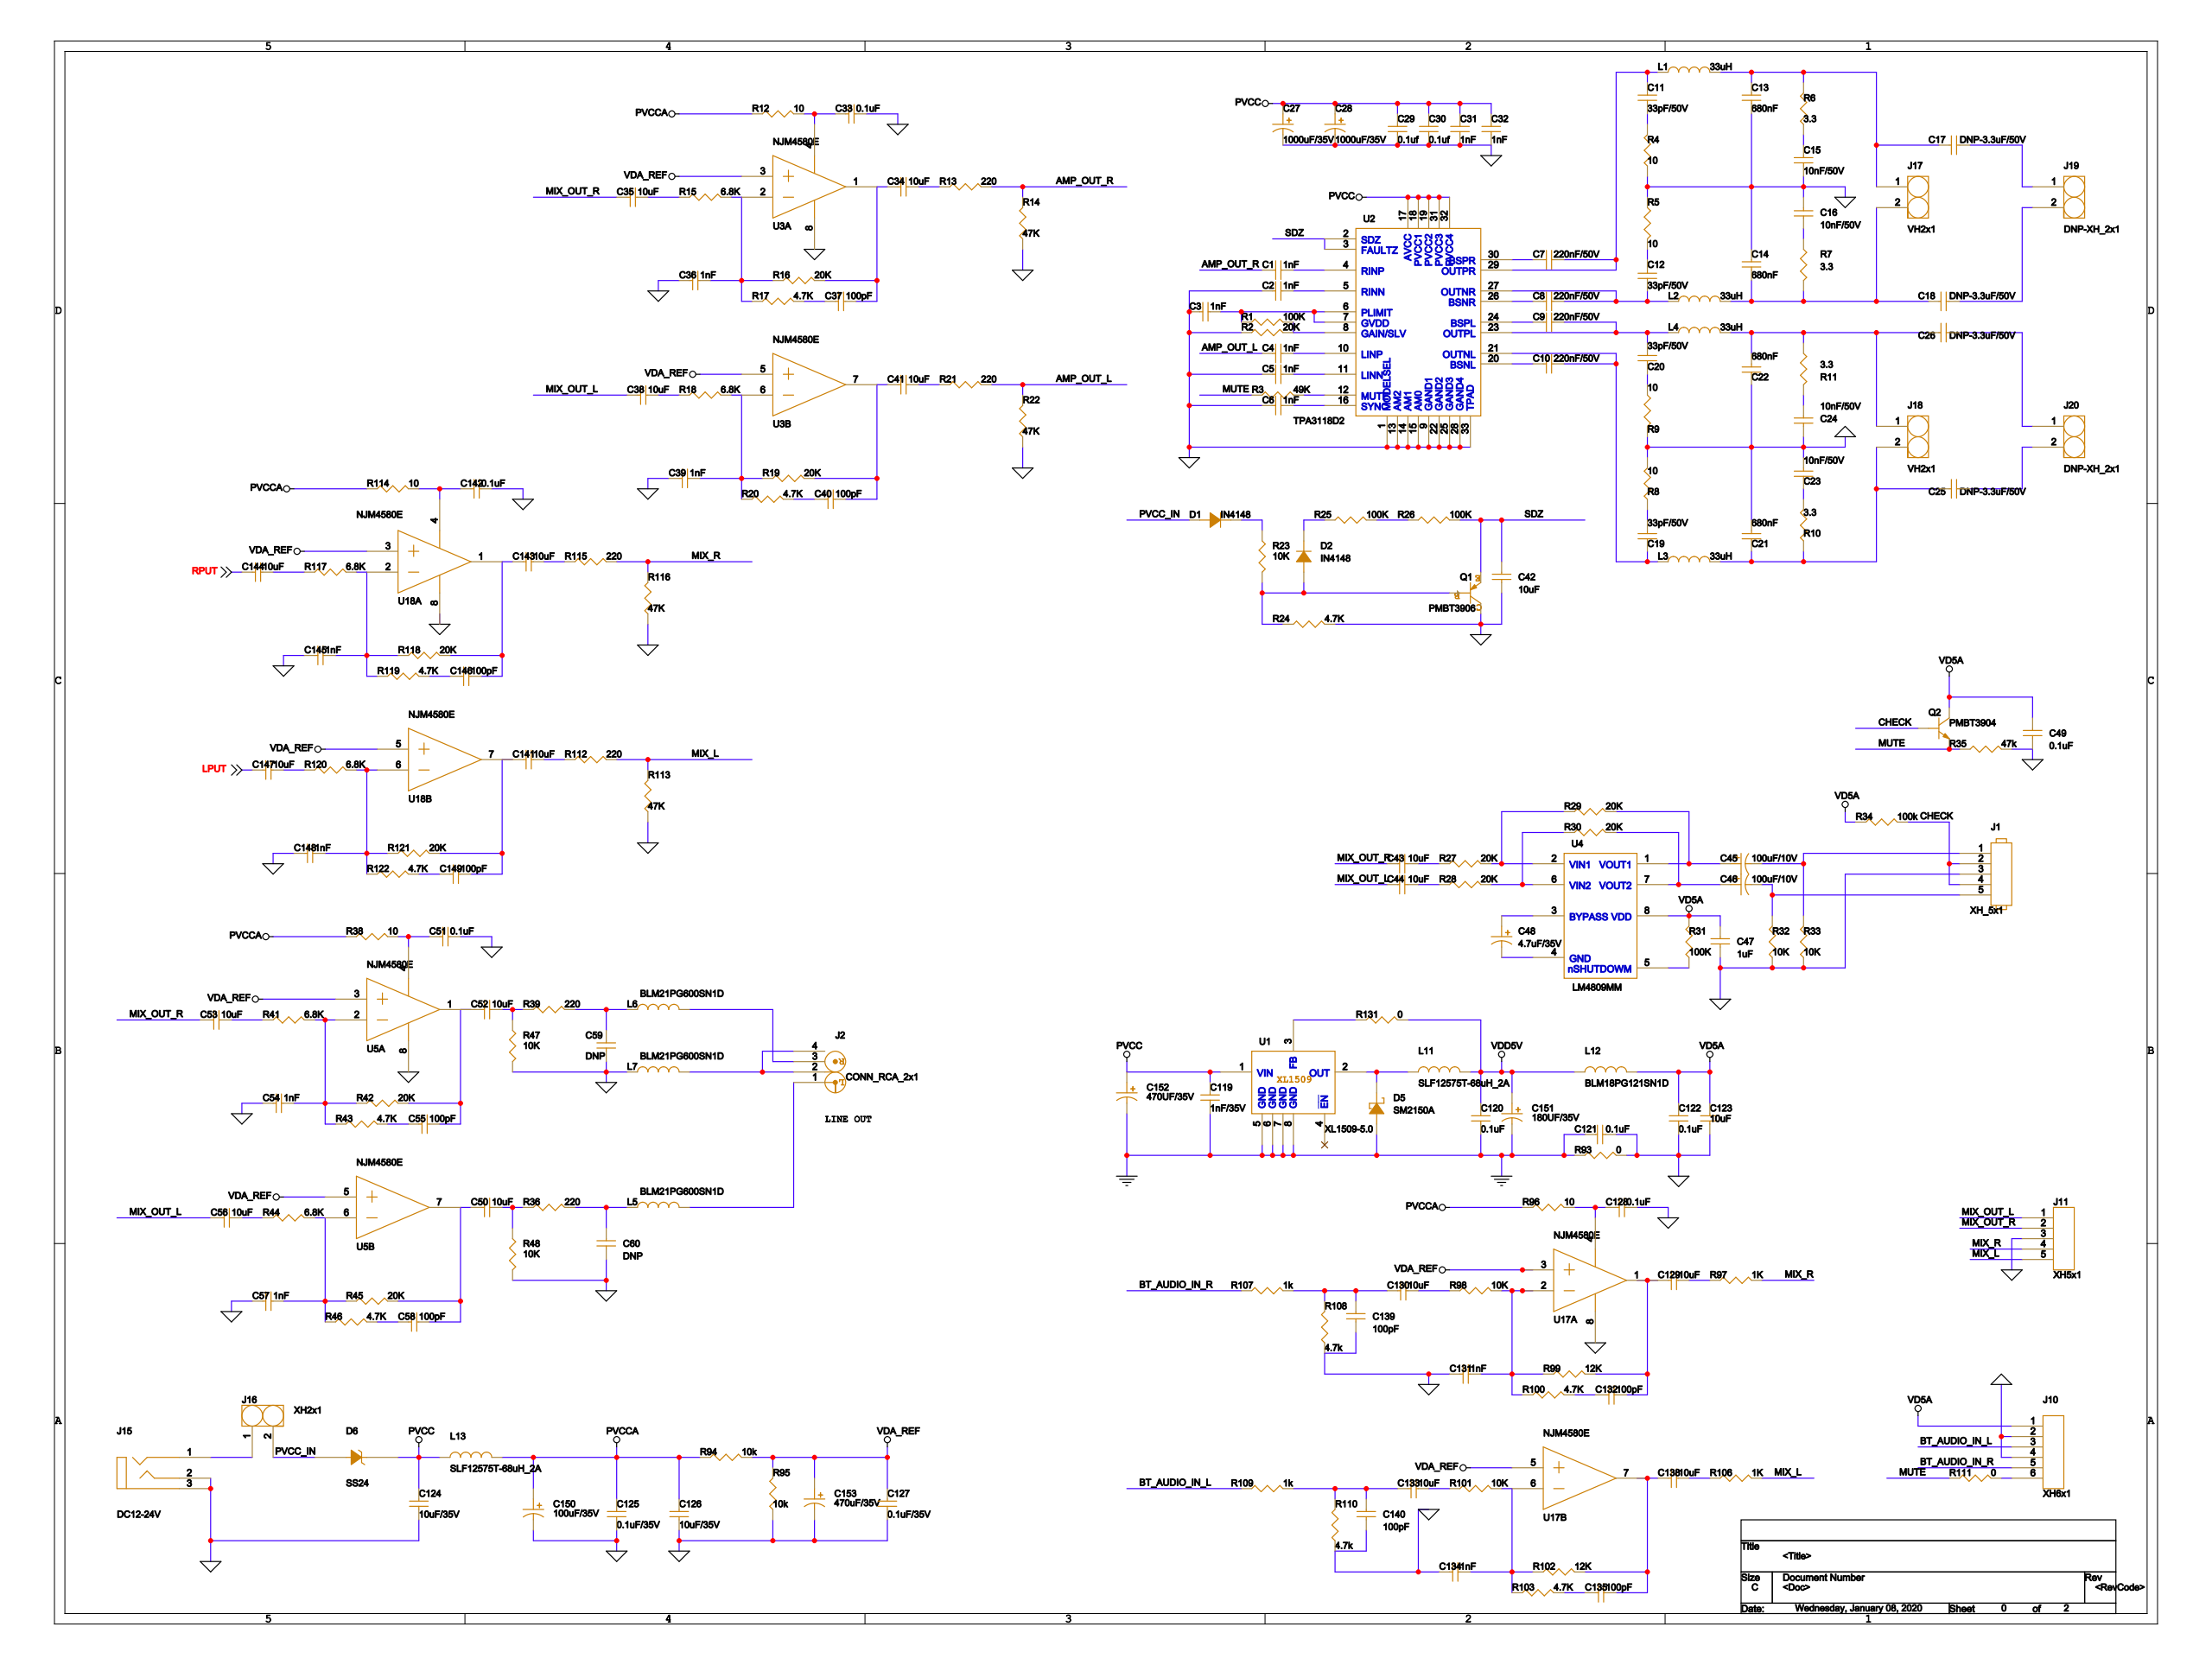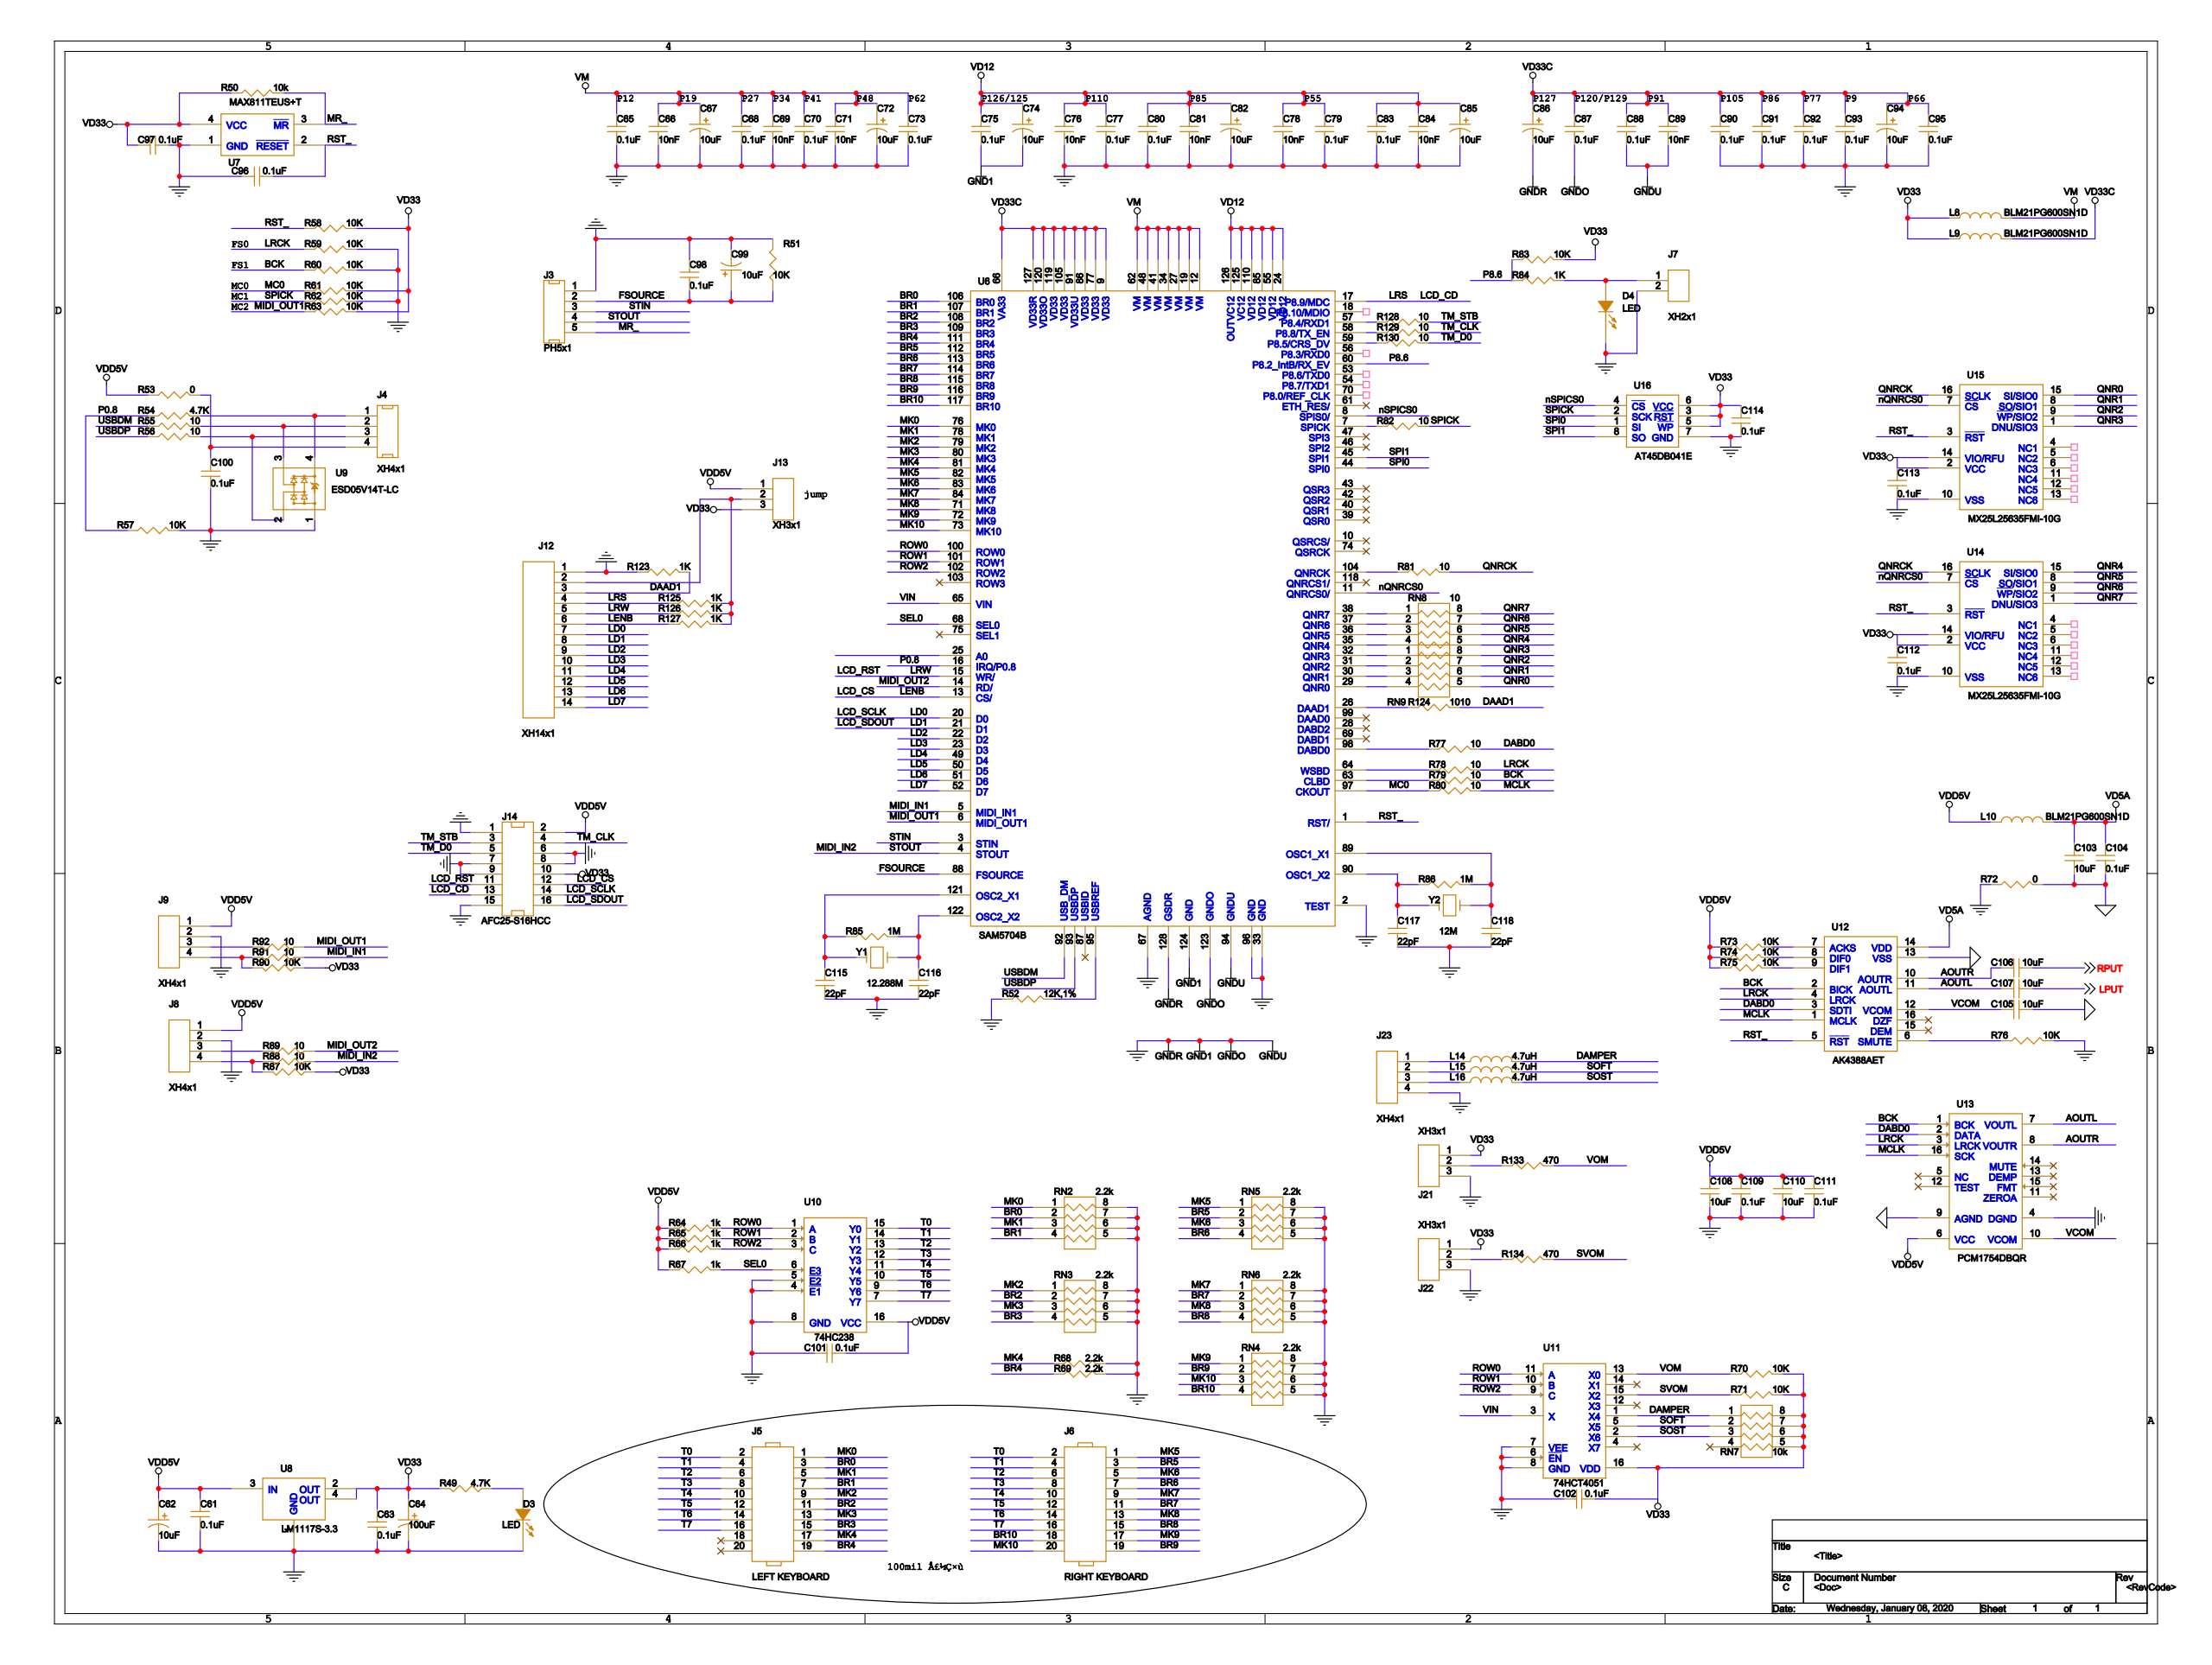Circuit board | Cadence Allegro | 355 parts | 259 nets
Bill of materials:
SYM_NAME,COMP_DEVICE_TYPE,COMP_VALUE,COMP_TOL,COMP_CLASS,REFDES
C0603,CAP NP_C0603_1NF,1nF,,IC,C1
C0603,CAP NP_C0603_1NF,1nF,,IC,C2
C0603,CAP NP_C0603_1NF,1nF,,IC,C3
C0603,CAP NP_C0603_1NF,1nF,,IC,C4
C0603,CAP NP_C0603_1NF,1nF,,IC,C5
C0603,CAP NP_C0603_1NF,1nF,,IC,C6
C0603,CAP NP_C0603_220NF/50V,220nF/50V,,IC,C7
C0603,CAP NP_C0603_220NF/50V,220nF/50V,,IC,C8
C0603,CAP NP_C0603_220NF/50V,220nF/50V,,IC,C9
C0603,CAP NP_C0603_220NF/50V,220nF/50V,,IC,C10
C0603,CAP NP_C0603_33PF/50V,33pF/50V,,IC,C11
C0603,CAP NP_C0603_33PF/50V,33pF/50V,,IC,C12
C0603,CAP NP_C0603_680NF,680nF,,IC,C13
C0603,CAP NP_C0603_680NF,680nF,,IC,C14
C0603,CAP NP_C0603_10NF/50V,10nF/50V,,IC,C15
C0603,CAP NP_C0603_10NF/50V,10nF/50V,,IC,C16
C0603,CAP NP_C0603_DNP-3.3UF/50V,DNP-3.3uF/50V,,IC,C17
C0603,CAP NP_C0603_DNP-3.3UF/50V,DNP-3.3uF/50V,,IC,C18
C0603,CAP NP_C0603_33PF/50V,33pF/50V,,IC,C19
C0603,CAP NP_C0603_33PF/50V,33pF/50V,,IC,C20
C0603,CAP NP_C0603_680NF,680nF,,IC,C21
C0603,CAP NP_C0603_680NF,680nF,,IC,C22
C0603,CAP NP_C0603_10NF/50V,10nF/50V,,IC,C23
C0603,CAP NP_C0603_10NF/50V,10nF/50V,,IC,C24
C0603,CAP NP_C0603_DNP-3.3UF/50V,DNP-3.3uF/50V,,IC,C25
C0603,CAP NP_C0603_DNP-3.3UF/50V,DNP-3.3uF/50V,,IC,C26
CAP_13X20MM,CAP POL_CAP_13X20MM_1000UF/35V,1000uF/35V,,IC,C27
CAP_13X20MM,CAP POL_CAP_13X20MM_1000UF/35V,1000uF/35V,,IC,C28
C0603,CAP NP_C0603_0.1UF,0.1uF,,IC,C29
C0603,CAP NP_C0603_0.1UF,0.1uF,,IC,C30
C0603,CAP NP_C0603_1NF,1nF,,IC,C31
C0603,CAP NP_C0603_1NF,1nF,,IC,C32
C0603,CAP NP_C0603_0.1UF,0.1uF,,IC,C33
C0805,CAP NP_C0805_10UF,10uF,,IC,C34
C0805,CAP NP_C0805_10UF,10uF,,IC,C35
C0603,CAP NP_C0603_1NF,1nF,,IC,C36
C0603,CAP NP_C0603_100PF,100pF,,IC,C37
C0805,CAP NP_C0805_10UF,10uF,,IC,C38
C0603,CAP NP_C0603_1NF,1nF,,IC,C39
C0603,CAP NP_C0603_100PF,100pF,,IC,C40
C0805,CAP NP_C0805_10UF,10uF,,IC,C41
C0805,CAP NP_C0805_10UF,10uF,,IC,C42
C0805,CAP NP_C0805_10UF,10uF,,IC,C43
C0805,CAP NP_C0805_10UF,10uF,,IC,C44
CAP_6P3X11MM,CAP POL_CAP_6P3X11MM_100UF/10V,100uF/10V,,IC,C45
CAP_6P3X11MM,CAP POL_CAP_6P3X11MM_100UF/10V,100uF/10V,,IC,C46
C0603,CAP NP_C0603_1UF,1uF,,IC,C47
CAP_4X7MM,CAP POL_CAP_4X7MM_4.7UF/35V,4.7uF/35V,,IC,C48
C0603,CAP NP_C0603_0.1UF,0.1uF,,IC,C49
C0805,CAP NP_C0805_10UF,10uF,,IC,C50
C0603,CAP NP_C0603_0.1UF,0.1uF,,IC,C51
C0805,CAP NP_C0805_10UF,10uF,,IC,C52
C0805,CAP NP_C0805_10UF,10uF,,IC,C53
C0603,CAP NP_C0603_1NF,1nF,,IC,C54
C0603,CAP NP_C0603_100PF,100pF,,IC,C55
C0805,CAP NP_C0805_10UF,10uF,,IC,C56
C0603,CAP NP_C0603_1NF,1nF,,IC,C57
C0603,CAP NP_C0603_100PF,100pF,,IC,C58
C0603,CAP NP_C0603_DNP,DNP,,IC,C59
C0603,CAP NP_C0603_DNP,DNP,,IC,C60
C0603,CAP NP_C0603_0.1UF,0.1uF,,IC,C61
C0805,CAP POL_C0805_10UF,10uF,,IC,C62
C0603,CAP NP_C0603_0.1UF,0.1uF,,IC,C63
CAP_6P3X11MM,CAP POL_CAP_6P3X11MM_100UF,100uF,,IC,C64
C0603,CAP NP_C0603_0.1UF,0.1uF,,IC,C65
C0603,CAP NP_C0603_10NF,10nF,,IC,C66
C0805,CAP POL_C0805_10UF,10uF,,IC,C67
C0603,CAP NP_C0603_0.1UF,0.1uF,,IC,C68
C0603,CAP NP_C0603_10NF,10nF,,IC,C69
C0603,CAP NP_C0603_0.1UF,0.1uF,,IC,C70
C0603,CAP NP_C0603_10NF,10nF,,IC,C71
C0805,CAP POL_C0805_10UF,10uF,,IC,C72
C0603,CAP NP_C0603_0.1UF,0.1uF,,IC,C73
C0805,CAP POL_C0805_10UF,10uF,,IC,C74
C0603,CAP NP_C0603_0.1UF,0.1uF,,IC,C75
C0603,CAP NP_C0603_10NF,10nF,,IC,C76
C0603,CAP NP_C0603_0.1UF,0.1uF,,IC,C77
C0603,CAP NP_C0603_10NF,10nF,,IC,C78
C0603,CAP NP_C0603_0.1UF,0.1uF,,IC,C79
C0603,CAP NP_C0603_0.1UF,0.1uF,,IC,C80
C0603,CAP NP_C0603_10NF,10nF,,IC,C81
C0805,CAP POL_C0805_10UF,10uF,,IC,C82
C0603,CAP NP_C0603_0.1UF,0.1uF,,IC,C83
C0603,CAP NP_C0603_10NF,10nF,,IC,C84
C0805,CAP POL_C0805_10UF,10uF,,IC,C85
C0805,CAP POL_C0805_10UF,10uF,,IC,C86
C0603,CAP NP_C0603_0.1UF,0.1uF,,IC,C87
C0603,CAP NP_C0603_0.1UF,0.1uF,,IC,C88
C0603,CAP NP_C0603_10NF,10nF,,IC,C89
C0603,CAP NP_C0603_0.1UF,0.1uF,,IC,C90
C0603,CAP NP_C0603_0.1UF,0.1uF,,IC,C91
C0603,CAP NP_C0603_0.1UF,0.1uF,,IC,C92
C0603,CAP NP_C0603_0.1UF,0.1uF,,IC,C93
C0805,CAP POL_C0805_10UF,10uF,,IC,C94
C0603,CAP NP_C0603_0.1UF,0.1uF,,IC,C95
C0603,CAP NP_C0603_0.1UF,0.1uF,,IC,C96
C0603,CAP NP_C0603_0.1UF,0.1uF,,IC,C97
C0603,CAP NP_C0603_0.1UF,0.1uF,,IC,C98
C0805,CAP POL_C0805_10UF,10uF,,IC,C99
C0603,CAP NP_C0603_0.1UF,0.1uF,,IC,C100
C0603,CAP NP_C0603_0.1UF,0.1uF,,IC,C101
C0603,CAP NP_C0603_0.1UF,0.1uF,,IC,C102
C0805,CAP NP_C0805_10UF,10uF,,IC,C103
C0603,CAP NP_C0603_0.1UF,0.1uF,,IC,C104
C0805,CAP NP_C0805_10UF,10uF,,IC,C105
C0805,CAP NP_C0805_10UF,10uF,,IC,C106
C0805,CAP NP_C0805_10UF,10uF,,IC,C107
C0805,CAP NP_C0805_10UF,10uF,,IC,C108
C0603,CAP NP_C0603_0.1UF,0.1uF,,IC,C109
C0805,CAP NP_C0805_10UF,10uF,,IC,C110
C0603,CAP NP_C0603_0.1UF,0.1uF,,IC,C111
C0603,CAP NP_C0603_0.1UF,0.1uF,,IC,C112
C0603,CAP NP_C0603_0.1UF,0.1uF,,IC,C113
C0603,CAP NP_C0603_0.1UF,0.1uF,,IC,C114
C0603,CAP NP_C0603_22PF,22pF,,IC,C115
C0603,CAP NP_C0603_22PF,22pF,,IC,C116
C0603,CAP NP_C0603_22PF,22pF,,IC,C117
C0603,CAP NP_C0603_22PF,22pF,,IC,C118
C0603,CAP NP_C0603_1NF/35V,1nF/35V,,IC,C119
C0603,CAP NP_C0603_0.1UF,0.1uF,,IC,C120
C0603,CAP NP_C0603_0.1UF,0.1uF,,IC,C121
C0603,CAP NP_C0603_0.1UF,0.1uF,,IC,C122
C0805,CAP NP_C0805_10UF,10uF,,IC,C123
C0805,CAP NP_C0805_10UF/35V,10uF/35V,,IC,C124
C0603,CAP NP_C0603_0.1UF/35V,0.1uF/35V,,IC,C125
C0805,CAP NP_C0805_10UF/35V,10uF/35V,,IC,C126
C0603,CAP NP_C0603_0.1UF/35V,0.1uF/35V,,IC,C127
C0603,CAP NP_C0603_0.1UF,0.1uF,,IC,C128
C0805,CAP NP_C0805_10UF,10uF,,IC,C129
C0805,CAP NP_C0805_10UF,10uF,,IC,C130
C0603,CAP NP_C0603_1NF,1nF,,IC,C131
C0603,CAP NP_C0603_100PF,100pF,,IC,C132
C0805,CAP NP_C0805_10UF,10uF,,IC,C133
C0603,CAP NP_C0603_1NF,1nF,,IC,C134
C0603,CAP NP_C0603_100PF,100pF,,IC,C135
C0805,CAP NP_C0805_10UF,10uF,,IC,C138
C0603,CAP NP_C0603_100PF,100pF,,IC,C139
C0603,CAP NP_C0603_100PF,100pF,,IC,C140
C0805,CAP NP_C0805_10UF,10uF,,IC,C141
C0603,CAP NP_C0603_0.1UF,0.1uF,,IC,C142
C0805,CAP NP_C0805_10UF,10uF,,IC,C143
C0805,CAP NP_C0805_10UF,10uF,,IC,C144
C0603,CAP NP_C0603_1NF,1nF,,IC,C145
C0603,CAP NP_C0603_100PF,100pF,,IC,C146
C0805,CAP NP_C0805_10UF,10uF,,IC,C147
C0603,CAP NP_C0603_1NF,1nF,,IC,C148
C0603,CAP NP_C0603_100PF,100pF,,IC,C149
CAP_6P3X11MM,CAP POL_CAP_6P3X11MM_100UF/35V,100uF/35V,,IC,C150
CAP_6P3X11MM,CAP POL_CAP_6P3X11MM_180UF/35V,180UF/35V,,IC,C151
CAP_10X17MM,CAP POL_CAP_10X17MM_470UF/35V,470UF/35V,,IC,C152
CAP_10X17MM,CAP POL_CAP_10X17MM_470UF/35V,470UF/35V,,IC,C153
SOD-123,DIODE_SOD-123_IN4148,IN4148,,IC,D1
SOD-123,DIODE_SOD-123_IN4148,IN4148,,IC,D2
LED0805,LED_0_LED0805_LED,LED,,IC,D3
LED0805,LED_0_LED0805_LED,LED,,IC,D4
SMA-FL,SGL41/SM_SMA-FL_SM2150A,SM2150A,,IC,D5
DO-214AC_5P28X2P9M,ICL8069/SO_0_DO-214AC_5P28X2P9M,SS24,,IC,D6
XH-5A,HEADER 5_XH-5A_XH_5X1,XH_5x1,,IC,J1
XH-4A,CONN_RCA_0_XH-4A_CONN_RCA_2X1,CONN_RCA_2x1,,IC,J2
PH-5A,CONN RECT 5_PH-5A_PH5X1,PH5x1,,IC,J3
XH-4A,CONN PCB 4-R_XH-4A_XH4X1,XH4x1,,IC,J4
IDC10X2,HEADER 10X2_IDC10X2_LEFT KEYBOA,LEFT KEYBOARD,,IC,J5
IDC10X2,HEADER 10X2_IDC10X2_RIGHT KEYBO,RIGHT KEYBOARD,,IC,J6
XH-2A,CON2_XH-2A_XH2X1,XH2x1,,IC,J7
XH254_4_V,CON4_XH254_4_V_XH4X1,XH4x1,,IC,J8
XH254_4_V,CON4_XH254_4_V_XH4X1,XH4x1,,IC,J9
XH-6A,CON6_XH-6A_XH6X1,XH6x1,,IC,J10
XH-5A,CON5_XH-5A_XH5X1,XH5x1,,IC,J11
XH254_14_V,CON14_XH254_14_V_XH14X1,XH14x1,,IC,J12
XH-3A,CON3_XH-3A_XH3X1,XH3x1,,IC,J13
FPC_1P25MM16P,CONN PCB 8X2-R_FPC_1P25MM16P_AF,AFC25-S16HCC,,IC,J14
DC-0055P5-2P0MM,PHONEJACK STEREO_DC-0055P5-2P0M,DC12-24V,,IC,J15
XH-2A,XH2X1_XH-2A_XH2X1,XH2x1,,IC,J16
VH-2A,XH2X1_VH-2A_VH2X1,VH2x1,,IC,J17
VH-2A,XH2X1_VH-2A_VH2X1,VH2x1,,IC,J18
XH-2A,XH2X1_XH-2A_DNP-XH_2X1,DNP-XH_2x1,,IC,J19
XH-2A,XH2X1_XH-2A_DNP-XH_2X1,DNP-XH_2x1,,IC,J20
XH-3A,CON3_XH-3A_XH3X1,XH3x1,,IC,J21
XH-3A,CON3_XH-3A_XH3X1,XH3x1,,IC,J22
XH254_4_V,CON4_XH254_4_V_XH4X1,XH4x1,,IC,J23
L_12P5X12P5X7P5MM,INDUCTOR_L_12P5X12P5X7P5MM_33UH,33uH,,IC,L1
L_12P5X12P5X7P5MM,INDUCTOR_L_12P5X12P5X7P5MM_33UH,33uH,,IC,L2
L_12P5X12P5X7P5MM,INDUCTOR_L_12P5X12P5X7P5MM_33UH,33uH,,IC,L3
L_12P5X12P5X7P5MM,INDUCTOR_L_12P5X12P5X7P5MM_33UH,33uH,,IC,L4
L0603,INDUCTOR_L0603_ BLM21PG600SN1D,BLM21PG600SN1D,,IC,L5
L0603,INDUCTOR_L0603_ BLM21PG600SN1D,BLM21PG600SN1D,,IC,L6
L0603,INDUCTOR_L0603_ BLM21PG600SN1D,BLM21PG600SN1D,,IC,L7
L0805,INDUCTOR_L0805_ BLM21PG600SN1D,BLM21PG600SN1D,,IC,L8
L0805,INDUCTOR_L0805_ BLM21PG600SN1D,BLM21PG600SN1D,,IC,L9
L0805,INDUCTOR_L0805_ BLM21PG600SN1D,BLM21PG600SN1D,,IC,L10
L_12P5X12P5X7P5MM,INDUCTOR_L_12P5X12P5X7P5MM_SLF1,SLF12575T-68uH_2A,,IC,L11
L0603,INDUCTOR_L0603_BLM18PG121SN1D,BLM18PG121SN1D,,IC,L12
L_12P5X12P5X7P5MM,INDUCTOR_L_12P5X12P5X7P5MM_SLF1,SLF12575T-68uH_2A,,IC,L13
L0805,INDUCTOR_L0805_4.7UH,4.7uH,,IC,L14
L0805,INDUCTOR_L0805_4.7UH,4.7uH,,IC,L15
L0805,INDUCTOR_L0805_4.7UH,4.7uH,,IC,L16
SOT-23,PMBT3906_0_SOT-23_PMBT3906,PMBT3906,,IC,Q1
SOT-23,PMBT3904_0_SOT-23_PMBT3904,PMBT3904,,IC,Q2
R0603,R_R0603_100K,100K,,IC,R1
R0603,R_R0603_20K,20K,,IC,R2
R0603,R_R0603_49K,49K,,IC,R3
R0603,R_R0603_10,10,,IC,R4
R0603,R_R0603_10,10,,IC,R5
R0603,R_R0603_3.3,3.3,,IC,R6
R0603,R_R0603_3.3,3.3,,IC,R7
R0603,R_R0603_10,10,,IC,R8
R0603,R_R0603_10,10,,IC,R9
R0603,R_R0603_3.3,3.3,,IC,R10
R0603,R_R0603_3.3,3.3,,IC,R11
R0603,R_R0603_10,10,,IC,R12
R0603,R_R0603_220,220,,IC,R13
R0603,R_R0603_47K,47K,,IC,R14
R0603,R_R0603_6.8K,6.8K,,IC,R15
R0603,R_R0603_20K,20K,,IC,R16
R0603,R_R0603_4.7K,4.7K,,IC,R17
R0603,R_R0603_6.8K,6.8K,,IC,R18
R0603,R_R0603_20K,20K,,IC,R19
R0603,R_R0603_4.7K,4.7K,,IC,R20
R0603,R_R0603_220,220,,IC,R21
R0603,R_R0603_47K,47K,,IC,R22
R0603,R_R0603_10K,10K,,IC,R23
R0603,R_R0603_4.7K,4.7K,,IC,R24
R0603,R_R0603_100K,100K,,IC,R25
R0603,R_R0603_100K,100K,,IC,R26
R0603,R_R0603_20K,20K,,IC,R27
R0603,R_R0603_20K,20K,,IC,R28
R0603,R_R0603_20K,20K,,IC,R29
R0603,R_R0603_20K,20K,,IC,R30
R0603,R_R0603_100K,100K,,IC,R31
R0603,R_R0603_10K,10K,,IC,R32
R0603,R_R0603_10K,10K,,IC,R33
R0603,R_R0603_100K,100K,,IC,R34
R0603,R_R0603_47K,47K,,IC,R35
R0603,R_R0603_220,220,,IC,R36
R0603,R_R0603_10,10,,IC,R38
R0603,R_R0603_220,220,,IC,R39
R0603,R_R0603_6.8K,6.8K,,IC,R41
R0603,R_R0603_20K,20K,,IC,R42
R0603,R_R0603_4.7K,4.7K,,IC,R43
R0603,R_R0603_6.8K,6.8K,,IC,R44
R0603,R_R0603_20K,20K,,IC,R45
R0603,R_R0603_4.7K,4.7K,,IC,R46
R0603,R_R0603_10K,10K,,IC,R47
R0603,R_R0603_10K,10K,,IC,R48
R0603,R_R0603_4.7K,4.7K,,IC,R49
R0603,R_R0603_10K,10K,,IC,R50
R0603,R_R0603_10K,10K,,IC,R51
R0603,"R_R0603_12K,1%","12K,1%",,IC,R52
R0603,R_R0603_0,0,,IC,R53
R0603,R_R0603_4.7K,4.7K,,IC,R54
R0603,R_R0603_10,10,,IC,R55
R0603,R_R0603_10,10,,IC,R56
R0603,R_R0603_10K,10K,,IC,R57
R0603,R_R0603_10K,10K,,IC,R58
R0603,R_R0603_10K,10K,,IC,R59
R0603,R_R0603_10K,10K,,IC,R60
R0603,R_R0603_10K,10K,,IC,R61
R0603,R_R0603_10K,10K,,IC,R62
R0603,R_R0603_10K,10K,,IC,R63
R0603,R_R0603_1K,1K,,IC,R64
R0603,R_R0603_1K,1K,,IC,R65
R0603,R_R0603_1K,1K,,IC,R66
R0603,R_R0603_1K,1K,,IC,R67
R0603,R_R0603_2.2K,2.2k,,IC,R68
R0603,R_R0603_2.2K,2.2k,,IC,R69
R0603,R_R0603_10K,10K,,IC,R70
R0603,R_R0603_10K,10K,,IC,R71
R0603,R_R0603_0,0,,IC,R72
R0603,R_R0603_10K,10K,,IC,R73
R0603,R_R0603_10K,10K,,IC,R74
R0603,R_R0603_10K,10K,,IC,R75
R0603,R_R0603_10K,10K,,IC,R76
R0603,R_R0603_10,10,,IC,R77
R0603,R_R0603_10,10,,IC,R78
R0603,R_R0603_10,10,,IC,R79
R0603,R_R0603_10,10,,IC,R80
R0603,R_R0603_10,10,,IC,R81
R0603,R_R0603_10,10,,IC,R82
R0603,R_R0603_10K,10K,,IC,R83
R0603,R_R0603_1K,1K,,IC,R84
R0603,R_R0603_1M,1M,,IC,R85
R0603,R_R0603_1M,1M,,IC,R86
R0603,R_R0603_10K,10K,,IC,R87
R0603,R_R0603_10,10,,IC,R88
R0603,R_R0603_10,10,,IC,R89
R0603,R_R0603_10K,10K,,IC,R90
R0603,R_R0603_10,10,,IC,R91
R0603,R_R0603_10,10,,IC,R92
R0603,R_R0603_0,0,,IC,R93
R0603,R_R0603_10K,10K,,IC,R94
R0603,R_R0603_10K,10K,,IC,R95
R0603,R_R0603_10,10,,IC,R96
R0603,R_R0603_1K,1K,,IC,R97
R0603,R_R0603_10K,10K,,IC,R98
R0603,R_R0603_12K,12K,,IC,R99
R0603,R_R0603_4.7K,4.7K,,IC,R100
R0603,R_R0603_10K,10K,,IC,R101
R0603,R_R0603_12K,12K,,IC,R102
R0603,R_R0603_4.7K,4.7K,,IC,R103
R0603,R_R0603_1K,1K,,IC,R106
R0603,R_R0603_1K,1K,,IC,R107
R0603,R_R0603_4.7K,4.7K,,IC,R108
R0603,R_R0603_1K,1K,,IC,R109
R0603,R_R0603_4.7K,4.7K,,IC,R110
R0603,R_R0603_0,0,,IC,R111
R0603,R_R0603_220,220,,IC,R112
R0603,R_R0603_47K,47K,,IC,R113
R0603,R_R0603_10,10,,IC,R114
R0603,R_R0603_220,220,,IC,R115
R0603,R_R0603_47K,47K,,IC,R116
R0603,R_R0603_6.8K,6.8K,,IC,R117
R0603,R_R0603_20K,20K,,IC,R118
R0603,R_R0603_4.7K,4.7K,,IC,R119
R0603,R_R0603_6.8K,6.8K,,IC,R120
R0603,R_R0603_20K,20K,,IC,R121
R0603,R_R0603_4.7K,4.7K,,IC,R122
R0603,R_R0603_1K,1K,,IC,R123
R0603,R_R0603_10,10,,IC,R124
R0603,R_R0603_1K,1K,,IC,R125
R0603,R_R0603_1K,1K,,IC,R126
R0603,R_R0603_1K,1K,,IC,R127
R0603,R_R0603_10,10,,IC,R128
R0603,R_R0603_10,10,,IC,R129
R0603,R_R0603_10,10,,IC,R130
R0603,R_R0603_0,0,,IC,R131
R0603,R_R0603_470,470,,IC,R133
R0603,R_R0603_470,470,,IC,R134
RN0603,RESISTOR DIP 4_RN0603_2.2K,2.2k,,IC,RN2
RN0603,RESISTOR DIP 4_RN0603_2.2K,2.2k,,IC,RN3
RN0603,RESISTOR DIP 4_RN0603_2.2K,2.2k,,IC,RN4
RN0603,RESISTOR DIP 4_RN0603_2.2K,2.2k,,IC,RN5
RN0603,RESISTOR DIP 4_RN0603_2.2K,2.2k,,IC,RN6
RN0603,RESISTOR DIP 4_RN0603_10K,10k,,IC,RN7
RN0603,RESISTOR DIP 4_RN0603_10,10,,IC,RN8
RN0603,RESISTOR DIP 4_RN0603_10,10,,IC,RN9
SO8,XL1509-5_1.0_SO8_XL1509-5.0,XL1509-5.0,,IC,U1
DAP-32,TPA3118D2_DAP-32_TPA3118D2,TPA3118D2,,IC,U2
SO8,LMV358_SO8_NJM4580E,NJM4580E,,IC,U3
TSSOP8_0P65M_3X5M,LM4809MM_TSSOP8_0P65M_3X5M_LM48,LM4809MM,,IC,U4
SO8,LMV358_SO8_NJM4580E,NJM4580E,,IC,U5
LQFP128_P40,SAM5704B_5_LQFP128_P40_SAM5704B,SAM5704B,,IC,U6
SOT143_4,MAX811TEUS+T_0_SOT143_4_MAX811T,MAX811TEUS+T,,IC,U7
SOT223_4,LM1117S-3_0.3_SOT223_4_LM1117S-,LM1117S-3.3,,IC,U8
SOT143_4,ESD05V14T-LC_SOT143_4_ESD05V14T,ESD05V14T-LC,,IC,U9
SOIC16,74HC238_SOIC16_74HC238,74HC238,,IC,U10
SOIC16,74HCT4051_SOIC16_74HCT4051,74HCT4051,,IC,U11
TSSOP16,AK4388AET_TSSOP16_AK4388AET,AK4388AET,,IC,U12
SSOP16,PCM1754DBQR_SSOP16_PCM1754DBQR,PCM1754DBQR,,IC,U13
MX25L25635FMI-10G,MX25L25635FMI-10G_0_MX25L25635F,MX25L25635FMI-10G,,IC,U14
MX25L25635FMI-10G,MX25L25635FMI-10G_0_MX25L25635F,MX25L25635FMI-10G,,IC,U15
SO8,AT45DB041E_SO8_AT45DB041E,AT45DB041E,,IC,U16
SO8,LMV358_SO8_NJM4580E,NJM4580E,,IC,U17
SO8,LMV358_SO8_NJM4580E,NJM4580E,,IC,U18
XTALT_49S,CRYSTAL_XTALT_49S_12.288M,12.288M,,IC,Y1
XTALT_49S,CRYSTAL_XTALT_49S_12M,12M,,IC,Y2
Netlist (net: part-pin ...):
N03865: C13-1 C17-1 J17-1 L1-2 R6-2
N04851: C17-2 J19-1
N03930: C14-2 C18-1 J17-2 L2-2 R7-2
N04860: C18-2 J19-2
N05486: C21-1 C25-1 J18-2 L3-1 R10-2
N05726: C25-2 J20-2
N05526: C22-2 C26-1 J18-1 L4-1 R11-2
N05734: C26-2 J20-1
VD5A: C47-1 C49-1 C103-1 C104-1 C122-1 C123-1 J10-1 L10-2 L12-2 Q2-3 R31-2 R34-1 U4-8 U12-14
AGND: C2-2 C3-2 C5-2 C6-2 C13-2 C14-1 C15-2 C16-2 C21-2 C22-1 C23-2 C24-2 C27-2 C28-2 C29-2 C30-2 C31-2 C32-2 C33-1 C36-2 C39-2 C42-2 C47-2 C49-2 C51-1 C54-2 C57-2 C59-2 C60-2 C103-2 C104-2 C105-2 C121-2 C122-2 C123-2 C124-2 C125-2 C126-2 C127-2 C128-1 C131-2 C134-2 C139-2 C140-2 C142-1 C145-2 C148-2 C150-2 C153-2 J1-3 J10-2 J10-4 J11-3 J15-2 J15-3 L7-1 Q1-3 R2-1 R4-1 R5-1 R8-1 R9-1 R14-1 R22-1 R24-2 R32-1 R33-1 R35-2 R47-2 R48-2 R72-2 R93-2 R95-1 R108-1 R110-1 R113-1 R116-1 U2-1 U2-9 U2-13 U2-14 U2-15 U2-22 U2-25 U2-28 U2-33 U3-8 U5-8 U12-13 U13-9 U17-8 U18-8
VDD5V: C61-1 C62-1 C101-2 C108-1 C109-1 C110-1 C111-1 C120-1 C151-1 J8-1 J9-1 J13-1 J14-2 L10-1 L11-2 L12-1 R53-1 R64-1 R65-1 R66-1 R67-1 R73-1 R74-1 R75-1 R131-2 U8-3 U10-16 U13-6
N03382: C7-1 C11-1 L1-1 U2-29
N03378: C7-2 U2-30
N03493: C9-1 C20-1 L4-2 U2-23
N03489: C9-2 U2-24
N03538: C10-1 C19-1 L3-2 U2-21
N03534: C10-2 U2-20
N03433: C8-1 C12-1 L2-1 U2-27
N03429: C8-2 U2-26
GND: C61-2 C62-2 C63-2 C64-2 C65-2 C66-2 C67-2 C68-2 C69-2 C70-2 C71-2 C72-2 C73-2 C74-2 C75-2 C76-2 C77-2 C78-2 C79-2 C80-2 C81-2 C82-2 C83-2 C84-2 C85-2 C86-2 C87-2 C88-2 C89-2 C90-2 C91-2 C92-2 C93-2 C94-2 C95-2 C96-1 C97-2 C98-1 C99-2 C100-1 C101-1 C102-1 C108-2 C109-2 C110-2 C111-2 C112-2 C113-2 C114-2 C115-2 C116-2 C117-2 C118-2 C119-2 C120-2 C121-1 C151-2 C152-2 D3-2 D4-2 D5-1 J3-1 J7-2 J8-2 J9-2 J12-1 J14-1 J14-6 J14-7 J14-8 J14-9 J14-15 J21-3 J22-3 J23-4 R51-2 R52-1 R57-2 R59-2 R60-2 R62-2 R68-2 R69-2 R72-1 R76-2 R93-1 R123-1 RN2-5 RN2-6 RN2-7 RN2-8 RN3-5 RN3-6 RN3-7 RN3-8 RN4-5 RN4-6 RN4-7 RN4-8 RN5-5 RN5-6 RN5-7 RN5-8 RN6-5 RN6-6 RN6-7 RN6-8 U1-5 U1-6 U1-7 U1-8 U6-2 U6-33 U6-67 U6-94 U6-96 U6-123 U6-124 U6-128 U7-1 U8-1 U9-1 U10-4 U10-5 U10-8 U11-6 U11-7 U11-8 U13-4 U14-10 U15-10 U16-7
N38386: D3-1 R49-1
N131746: D4-1 J7-1 R84-2
N378299: J23-1 L14-1
DAMPER: L14-2 RN7-3 U11-1
N378303: J23-2 L15-1
SOFT: L15-2 RN7-2 U11-5
N378307: J23-3 L16-1
SOST: L16-2 RN7-1 U11-2
N376097: J21-2 R133-1
VOM: R70-1 R133-2 U11-13
N377289: J22-2 R134-1
SVOM: R71-1 R134-2 U11-15
PVCC: C27-1 C28-1 C29-1 C30-1 C31-1 C32-1 C119-1 C124-1 C152-1 D6-2 L13-1 U1-1 U2-17 U2-18 U2-19 U2-31 U2-32
SDZ: C42-1 Q1-2 R26-2 U2-2 U2-3
N02965: R1-2 R2-2 U2-8
N02895: C3-1 R1-1 U2-6 U2-7
N03104: C5-1 U2-11
N03064: C4-1 U2-10
N03153: R3-2 U2-12
N02865: C2-1 U2-5
N02833: C1-1 U2-4
N03197: C6-1 U2-16
PVCC_IN: D1-2 D6-1 J16-2
N14266: D2-2 Q1-1 R23-2 R24-1
CHECK: J1-2 J1-4 Q2-1 R34-2
MUTE: Q2-2 R3-1 R35-1 R111-1
N50853: J4-3 R56-2 U9-2
N50849: J4-2 R55-2 U9-3
N50733: J4-1 R54-2 U9-4
N237641: R131-1 U1-3
N159511: D5-2 L11-1 U1-2
N20707: C48-1 U4-3
N20711: C48-2 U4-4
N20396: R31-1 U4-5
N20155: R27-2 R29-1 U4-2
N20159: R28-2 R30-1 U4-6
N20259: C45-1 R29-2 U4-1
N20263: C46-1 R30-2 U4-7
NSPICS0: U6-8 U16-4
VD33: C63-1 C64-1 C97-1 C102-2 C112-1 C113-1 C114-1 J13-3 J14-10 J21-1 J22-1 L8-1 L9-1 R49-2 R50-1 R58-2 R61-2 R63-2 R70-2 R71-2 R83-2 R87-1 R90-1 RN7-5 RN7-6 RN7-7 RN7-8 U7-4 U8-2 U8-4 U11-16 U14-2 U14-14 U15-2 U15-14 U16-3 U16-5 U16-6
SPICK: R62-1 R82-2 U16-2
SPI0: U6-44 U16-1
SPI1: U6-45 U16-8
N100273: R73-2 U12-7
AOUTL: C107-1 U12-11 U13-7
AOUTR: C106-1 U12-10 U13-8
BCK: R60-1 R79-2 U12-2 U13-1
N100262: R74-2 U12-8
N100253: R75-2 U12-9
LRCK: R59-1 R78-2 U12-4 U13-3
MCLK: R80-2 U12-1 U13-16
RST_: C96-2 R58-1 U6-1 U7-2 U12-5 U14-3 U15-3
DABD0: R77-2 U12-3 U13-2
N101168: R76-1 U12-6
VCOM: C105-1 U12-12 U13-10
MR_: J3-5 R50-2 U7-3
ROW0: R64-2 U6-100 U10-1 U11-11
ROW1: R65-2 U6-101 U10-2 U11-10
ROW2: R66-2 U6-102 U10-3 U11-9
SEL0: R67-2 U6-68 U10-6
T0: J5-2 J6-2 U10-15
T1: J5-4 J6-4 U10-14
T2: J5-6 J6-6 U10-13
T3: J5-8 J6-8 U10-12
T4: J5-10 J6-10 U10-11
T5: J5-12 J6-12 U10-10
T6: J5-14 J6-14 U10-9
T7: J5-16 J6-16 U10-7
VIN: U6-65 U11-3
N139040: C115-1 R85-1 U6-121 Y1-1
N139047: C116-1 R85-2 U6-122 Y1-2
N140095: C117-1 R86-1 U6-90 Y2-1
N140075: C118-1 R86-2 U6-89 Y2-2
N12419: C39-1 R18-2 R19-1 R20-1 U3-6
AMP_OUT_R: C1-2 R13-2 R14-2
N168499: C131-1 R98-2 R99-1 R100-1 U17-2
N168699: C134-1 R101-2 R102-1 R103-1 U17-6
N188634: C145-1 R117-2 R118-1 R119-1 U18-2
N189044: C148-1 R120-2 R121-1 R122-1 U18-6
N10722: C36-1 R15-2 R16-1 R17-1 U3-2
AMP_OUT_L: C4-2 R21-2 R22-2
N25834: C54-1 R41-2 R42-1 R43-1 U5-2
N26244: C57-1 R44-2 R45-1 R46-1 U5-6
N50664: C100-2 J4-4 R53-2
N168391: C128-2 R96-2 U17-4
N188706: C142-2 R114-2 U18-4
N10267: C33-2 R12-2 U3-4
N25906: C51-2 R38-2 U5-4
VM: C65-1 C66-1 C67-1 C68-1 C69-1 C70-1 C71-1 C72-1 C73-1 L8-2 U6-12 U6-19 U6-27 U6-34 U6-41 U6-48 U6-62
VD12: C74-1 C75-1 C76-1 C77-1 C78-1 C79-1 C80-1 C81-1 C82-1 C83-1 C84-1 C85-1 U6-24 U6-55 U6-85 U6-110 U6-125 U6-126
VD33C: C86-1 C87-1 C88-1 C89-1 C90-1 C91-1 C92-1 C93-1 C94-1 C95-1 L9-2 U6-9 U6-66 U6-77 U6-86 U6-91 U6-105 U6-119 U6-120 U6-127
FSOURCE: C98-2 C99-1 J3-2 R51-1 U6-88
RPUT: C106-2 C144-2
LPUT: C107-2 C147-2
N168467: C129-1 R97-1
N168443: C129-2 C132-1 R99-2 U17-1
N168535: C130-1 R98-1
N168539: C130-2 C139-1 R107-2 R108-2
N168703: C133-1 R101-1
N171389: C133-2 C140-1 R109-2 R110-2
N168935: C138-1 R106-1
N168779: C135-1 C138-2 R102-2 U17-7
N188584: C141-1 R112-1
N188630: C141-2 C149-1 R121-2 U18-7
N188798: C143-1 R115-1
N188956: C143-2 C146-1 R118-2 U18-1
N188880: C144-1 R117-1
N189064: C147-1 R120-1
N10501: C34-1 R13-1
N11904: C34-2 C37-1 R16-2 U3-1
N11474: C35-1 R15-1
MIX_OUT_R: C35-2 C43-1 C53-2 J11-2
N12439: C38-1 R18-1
MIX_OUT_L: C38-2 C44-1 C56-2 J11-1
N13234: C41-1 R21-1
N12639: C40-1 C41-2 R19-2 U3-7
N20121: C43-2 R27-1
N20125: C44-2 R28-1
N25784: C50-1 R36-1 R48-1
N25830: C50-2 C58-1 R45-2 U5-7
N25998: C52-1 R39-1 R47-1
N26156: C52-2 C55-1 R42-2 U5-1
N26080: C53-1 R41-1
N26264: C56-1 R44-1
PVCCA: C125-1 C126-1 C150-1 L13-2 R12-1 R38-1 R94-1 R96-1 R114-1
VDA_REF: C127-1 C153-1 R94-2 R95-2 U3-3 U3-5 U5-3 U5-5 U17-3 U17-5 U18-3 U18-5
N12687: C40-2 R20-2
N12309: C37-2 R17-2
N168663: C132-2 R100-2
N168799: C135-2 R103-2
N189008: C146-2 R119-2
N189160: C149-2 R122-2
N26208: C55-2 R43-2
N26360: C58-2 R46-2
N04398: C15-1 R6-1
N05602: C24-1 R11-1
N04473: C16-1 R7-1
N05582: C23-1 R10-1
N03646: C11-2 R4-2
N03694: C12-2 R5-2
N05398: C20-2 R9-2
N05378: C19-2 R8-2
N20774: C45-2 J1-1 R33-2
N20767: C46-2 J1-5 R32-2
N26002: C59-1 L6-1 R39-2
N25788: C60-1 L5-1 R36-2
N14229: D1-1 R23-1
N14349: D2-1 R25-1
BT_AUDIO_IN_L: J10-3 R109-1
BT_AUDIO_IN_R: J10-5 R107-1
N179462: J10-6 R111-2
MIX_R: J11-4 R97-2 R115-2 R116-2
MIX_L: J11-5 R106-2 R112-2 R113-2
LD3: J12-10 U6-23
LD4: J12-11 U6-49
LD5: J12-12 U6-50
LD6: J12-13 U6-51
LD7: J12-14 U6-52
N190028: J12-2 J13-2 R125-2 R126-2 R127-2
DAAD1: J12-3 R123-2 R124-2
LCD_CD: J12-4 J14-13 R125-1 U6-17
LCD_RST: J12-5 J14-11 R126-1 U6-15
LCD_CS: J12-6 J14-12 R127-1 U6-13
LCD_SCLK: J12-7 J14-14 U6-20
LCD_SDOUT: J12-8 J14-16 U6-21
LD2: J12-9 U6-22
TM_STB: J14-3 R128-2
TM_CLK: J14-4 R129-2
TM_D0: J14-5 R130-2
N160976: J15-1 J16-1
N28654: J2-2 J2-4 L7-2
N28658: J2-1 L5-2
N28650: J2-3 L6-2
STIN: J3-3 U6-3
MIDI_IN2: J3-4 R88-1 U6-4
MK0: J5-1 RN2-4 U6-76
BR2: J5-11 RN3-3 U6-108
MK3: J5-13 RN3-2 U6-80
BR3: J5-15 RN3-1 U6-109
MK4: J5-17 R68-1 U6-81
BR4: J5-19 R69-1 U6-111
BR0: J5-3 RN2-3 U6-106
MK1: J5-5 RN2-2 U6-78
BR1: J5-7 RN2-1 U6-107
MK2: J5-9 RN3-4 U6-79
MK5: J6-1 RN5-1 U6-82
BR7: J6-11 RN6-2 U6-114
MK8: J6-13 RN6-3 U6-71
BR8: J6-15 RN6-4 U6-115
MK9: J6-17 RN4-1 U6-72
BR10: J6-18 RN4-4 U6-117
BR9: J6-19 RN4-2 U6-116
MK10: J6-20 RN4-3 U6-73
BR5: J6-3 RN5-2 U6-112
MK6: J6-5 RN5-3 U6-83
BR6: J6-7 RN5-4 U6-113
MK7: J6-9 RN6-1 U6-84
N141028: J8-3 R89-2
N142932: J8-4 R87-2 R88-2
N149706: J9-3 R92-2
N149590: J9-4 R90-2 R91-2
N14416: R25-2 R26-1
P0.8: R54-1 R57-1 U6-16
MC0: R61-1 R80-1 U6-97
MIDI_OUT1: R63-1 R92-1 U6-6
P8.6: R83-1 R84-1 U6-60
N193439: R124-1 U6-26
N205159: R128-1 U6-57
N205163: R129-1 U6-58
N205167: R130-1 U6-59
USBDM: R55-1 U6-92
USBDP: R56-1 U6-93
N108090: R77-1 U6-98
N108086: R78-1 U6-64
N108082: R79-1 U6-63
N111047: R81-1 U6-104
QNRCK: R81-2 U14-16 U15-16
N115336: R82-1 U6-7
MIDI_OUT2: R89-1 U6-14
MIDI_IN1: R91-1 U6-5
N49826: R52-2 U6-95
N110985: RN8-1 U6-38
N110981: RN8-2 U6-37
N110977: RN8-3 U6-36
N110973: RN8-4 U6-35
QNR4: RN8-5 U14-15
QNR5: RN8-6 U14-8
QNR6: RN8-7 U14-9
QNR7: RN8-8 U14-1
N110969: RN9-1 U6-32
N110965: RN9-2 U6-31
N110961: RN9-3 U6-30
N110957: RN9-4 U6-29
QNR0: RN9-5 U15-15
QNR1: RN9-6 U15-8
QNR2: RN9-7 U15-9
QNR3: RN9-8 U15-1
NQNRCS0: U6-11 U14-7 U15-7
N189947: U6-25